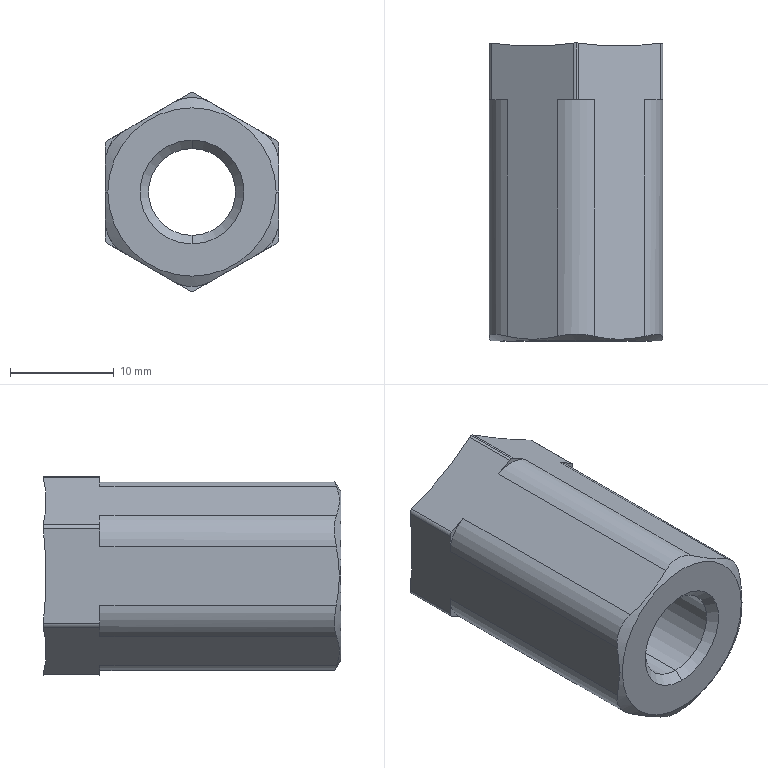Part | STEP file | _CMAZ40-N_a_n | 1 solid | 36 faces | box 16.7 x 28.679 x 19.129 mm | volume 5122 mm3 | cylinder 16 | plane 13 | cone 6 | spline 1 | commonest cylinder face diameters 1 x7 7 x7 8.376 x2
STEP:
#1=CARTESIAN_POINT('',(0.,4.188,4.188));
#2=VERTEX_POINT('',#1);
#3=CARTESIAN_POINT('',(0.,4.188,-4.188));
#4=VERTEX_POINT('',#3);
#5=CARTESIAN_POINT('',(0.,4.188,0.));
#6=DIRECTION('',(0.,-1.,0.));
#7=DIRECTION('',(0.,0.,-1.));
#8=AXIS2_PLACEMENT_3D('',#5,#6,#7);
#9=CIRCLE('',#8,4.188);
#10=EDGE_CURVE('',#2,#4,#9,.T.);
#11=ORIENTED_EDGE('',*,*,#10,.F.);
#12=CARTESIAN_POINT('',(0.,-22.388,4.188));
#13=VERTEX_POINT('',#12);
#14=CARTESIAN_POINT('',(0.,5.,4.188));
#15=DIRECTION('',(0.,-1.,0.));
#16=VECTOR('',#15,1000.);
#17=LINE('',#14,#16);
#18=EDGE_CURVE('',#2,#13,#17,.T.);
#19=ORIENTED_EDGE('',*,*,#18,.T.);
#20=CARTESIAN_POINT('',(0.,-22.388,-4.188));
#21=VERTEX_POINT('',#20);
#22=CARTESIAN_POINT('',(0.,-22.388,0.));
#23=DIRECTION('',(0.,1.,0.));
#24=DIRECTION('',(0.,0.,-1.));
#25=AXIS2_PLACEMENT_3D('',#22,#23,#24);
#26=CIRCLE('',#25,4.188);
#27=EDGE_CURVE('',#21,#13,#26,.T.);
#28=ORIENTED_EDGE('',*,*,#27,.F.);
#29=CARTESIAN_POINT('',(0.,5.,-4.188));
#30=DIRECTION('',(0.,-1.,0.));
#31=VECTOR('',#30,1000.);
#32=LINE('',#29,#31);
#33=EDGE_CURVE('',#4,#21,#32,.T.);
#34=ORIENTED_EDGE('',*,*,#33,.F.);
#35=EDGE_LOOP('',(#11,#19,#28,#34));
#36=FACE_OUTER_BOUND('',#35,.T.);
#37=CARTESIAN_POINT('',(0.,5.,0.));
#38=DIRECTION('',(0.,-1.,0.));
#39=DIRECTION('',(0.,0.,-1.));
#40=AXIS2_PLACEMENT_3D('',#37,#38,#39);
#41=CYLINDRICAL_SURFACE('',#40,4.188);
#42=ADVANCED_FACE('',(#36),#41,.F.);
#43=ORIENTED_EDGE('',*,*,#27,.T.);
#44=CARTESIAN_POINT('',(0.,-23.2,5.));
#45=VERTEX_POINT('',#44);
#46=CARTESIAN_POINT('',(0.,-23.2,5.));
#47=DIRECTION('',(0.,-0.7071,0.7071));
#48=VECTOR('',#47,1000.);
#49=LINE('',#46,#48);
#50=EDGE_CURVE('',#13,#45,#49,.T.);
#51=ORIENTED_EDGE('',*,*,#50,.T.);
#52=CARTESIAN_POINT('',(0.,-23.2,-5.));
#53=VERTEX_POINT('',#52);
#54=CARTESIAN_POINT('',(0.,-23.2,0.));
#55=DIRECTION('',(0.,1.,0.));
#56=DIRECTION('',(0.,0.,-1.));
#57=AXIS2_PLACEMENT_3D('',#54,#55,#56);
#58=CIRCLE('',#57,5.);
#59=EDGE_CURVE('',#53,#45,#58,.T.);
#60=ORIENTED_EDGE('',*,*,#59,.F.);
#61=CARTESIAN_POINT('',(0.,-23.2,-5.));
#62=DIRECTION('',(0.,-0.7071,-0.7071));
#63=VECTOR('',#62,1000.);
#64=LINE('',#61,#63);
#65=EDGE_CURVE('',#21,#53,#64,.T.);
#66=ORIENTED_EDGE('',*,*,#65,.F.);
#67=EDGE_LOOP('',(#43,#51,#60,#66));
#68=FACE_OUTER_BOUND('',#67,.T.);
#69=CARTESIAN_POINT('',(0.,-23.2,0.));
#70=DIRECTION('',(0.,-1.,0.));
#71=DIRECTION('',(0.,0.,-1.));
#72=AXIS2_PLACEMENT_3D('',#69,#70,#71);
#73=CONICAL_SURFACE('',#72,5.,0.7854);
#74=ADVANCED_FACE('',(#68),#73,.F.);
#75=ORIENTED_EDGE('',*,*,#10,.T.);
#76=CARTESIAN_POINT('',(0.,4.476,-4.476));
#77=VERTEX_POINT('',#76);
#78=CARTESIAN_POINT('',(0.,4.476,-4.476));
#79=DIRECTION('',(0.,0.7071,-0.7071));
#80=VECTOR('',#79,1000.);
#81=LINE('',#78,#80);
#82=EDGE_CURVE('',#4,#77,#81,.T.);
#83=ORIENTED_EDGE('',*,*,#82,.T.);
#84=CARTESIAN_POINT('',(0.,4.476,4.476));
#85=VERTEX_POINT('',#84);
#86=CARTESIAN_POINT('',(0.,4.476,0.));
#87=DIRECTION('',(0.,-1.,0.));
#88=DIRECTION('',(0.,0.,1.));
#89=AXIS2_PLACEMENT_3D('',#86,#87,#88);
#90=CIRCLE('',#89,4.476);
#91=EDGE_CURVE('',#85,#77,#90,.T.);
#92=ORIENTED_EDGE('',*,*,#91,.F.);
#93=CARTESIAN_POINT('',(0.,4.476,4.476));
#94=DIRECTION('',(0.,0.7071,0.7071));
#95=VECTOR('',#94,1000.);
#96=LINE('',#93,#95);
#97=EDGE_CURVE('',#2,#85,#96,.T.);
#98=ORIENTED_EDGE('',*,*,#97,.F.);
#99=EDGE_LOOP('',(#75,#83,#92,#98));
#100=FACE_OUTER_BOUND('',#99,.T.);
#101=CARTESIAN_POINT('',(0.,4.476,0.));
#102=DIRECTION('',(0.,1.,0.));
#103=DIRECTION('',(0.,0.,1.));
#104=AXIS2_PLACEMENT_3D('',#101,#102,#103);
#105=CONICAL_SURFACE('',#104,4.476,0.7854);
#106=ADVANCED_FACE('',(#100),#105,.F.);
#107=CARTESIAN_POINT('',(-8.1,-23.2,0.));
#108=VERTEX_POINT('',#107);
#109=CARTESIAN_POINT('',(8.1,-23.2,0.));
#110=VERTEX_POINT('',#109);
#111=CARTESIAN_POINT('',(0.,-23.2,0.));
#112=DIRECTION('',(0.,1.,0.));
#113=DIRECTION('',(-1.,0.,0.));
#114=AXIS2_PLACEMENT_3D('',#111,#112,#113);
#115=CIRCLE('',#114,8.1);
#116=EDGE_CURVE('',#108,#110,#115,.T.);
#117=ORIENTED_EDGE('',*,*,#116,.T.);
#118=CARTESIAN_POINT('',(8.35,-23.044,0.));
#119=VERTEX_POINT('',#118);
#120=CARTESIAN_POINT('',(9.106,-22.571,0.));
#121=DIRECTION('',(0.8481,0.5298,0.));
#122=VECTOR('',#121,1000.);
#123=LINE('',#120,#122);
#124=EDGE_CURVE('',#110,#119,#123,.T.);
#125=ORIENTED_EDGE('',*,*,#124,.T.);
#126=CARTESIAN_POINT('',(8.35,-22.758,2.8));
#127=VERTEX_POINT('',#126);
#128=CARTESIAN_POINT('',(8.35,-23.044,0.));
#129=CARTESIAN_POINT('',(8.35,-23.044,0.466));
#130=CARTESIAN_POINT('',(8.35,-23.019,0.9327));
#131=CARTESIAN_POINT('',(8.35,-22.923,1.867));
#132=CARTESIAN_POINT('',(8.35,-22.85,2.336));
#133=CARTESIAN_POINT('',(8.35,-22.758,2.8));
#134=B_SPLINE_CURVE_WITH_KNOTS('',3,(#128,#129,#130,#131,#132,#133),.UNSPECIFIED.,.F.,.F.,(4,2,4),(0.002807,0.004205,0.005602),.UNSPECIFIED.);
#135=EDGE_CURVE('',#119,#127,#134,.T.);
#136=ORIENTED_EDGE('',*,*,#135,.T.);
#137=CARTESIAN_POINT('',(6.6,-22.758,5.831));
#138=VERTEX_POINT('',#137);
#139=CARTESIAN_POINT('',(8.35,-22.758,2.8));
#140=CARTESIAN_POINT('',(8.35,-22.698,3.104));
#141=CARTESIAN_POINT('',(8.311,-22.653,3.404));
#142=CARTESIAN_POINT('',(8.193,-22.606,3.848));
#143=CARTESIAN_POINT('',(8.143,-22.595,3.995));
#144=CARTESIAN_POINT('',(8.026,-22.579,4.278));
#145=CARTESIAN_POINT('',(7.959,-22.575,4.416));
#146=CARTESIAN_POINT('',(7.729,-22.575,4.813));
#147=CARTESIAN_POINT('',(7.539,-22.591,5.062));
#148=CARTESIAN_POINT('',(7.108,-22.652,5.492));
#149=CARTESIAN_POINT('',(6.863,-22.698,5.679));
#150=CARTESIAN_POINT('',(6.6,-22.758,5.831));
#151=B_SPLINE_CURVE_WITH_KNOTS('',3,(#139,#140,#141,#142,#143,#144,#145,#146,#147,#148,#149,#150),.UNSPECIFIED.,.F.,.F.,(4,2,2,2,2,4),(0.,0.0009173,0.001376,0.001835,0.002752,0.003669),.UNSPECIFIED.);
#152=EDGE_CURVE('',#127,#138,#151,.T.);
#153=ORIENTED_EDGE('',*,*,#152,.T.);
#154=CARTESIAN_POINT('',(1.75,-22.758,8.631));
#155=VERTEX_POINT('',#154);
#156=CARTESIAN_POINT('',(6.6,-22.758,5.831));
#157=CARTESIAN_POINT('',(5.796,-22.943,6.296));
#158=CARTESIAN_POINT('',(4.989,-23.043,6.761));
#159=CARTESIAN_POINT('',(3.776,-23.044,7.462));
#160=CARTESIAN_POINT('',(3.371,-23.02,7.696));
#161=CARTESIAN_POINT('',(2.559,-22.923,8.164));
#162=CARTESIAN_POINT('',(2.153,-22.851,8.399));
#163=CARTESIAN_POINT('',(1.75,-22.758,8.631));
#164=B_SPLINE_CURVE_WITH_KNOTS('',3,(#156,#157,#158,#159,#160,#161,#162,#163),.UNSPECIFIED.,.F.,.F.,(4,2,2,4),(0.,0.002801,0.004202,0.005602),.UNSPECIFIED.);
#165=EDGE_CURVE('',#138,#155,#164,.T.);
#166=ORIENTED_EDGE('',*,*,#165,.T.);
#167=CARTESIAN_POINT('',(-1.75,-22.758,8.631));
#168=VERTEX_POINT('',#167);
#169=CARTESIAN_POINT('',(1.75,-22.758,8.631));
#170=CARTESIAN_POINT('',(1.487,-22.698,8.783));
#171=CARTESIAN_POINT('',(1.207,-22.653,8.9));
#172=CARTESIAN_POINT('',(0.7641,-22.606,9.019));
#173=CARTESIAN_POINT('',(0.6117,-22.595,9.05));
#174=CARTESIAN_POINT('',(0.3078,-22.579,9.09));
#175=CARTESIAN_POINT('',(0.1553,-22.575,9.1));
#176=CARTESIAN_POINT('',(-0.3037,-22.575,9.101));
#177=CARTESIAN_POINT('',(-0.6142,-22.591,9.059));
#178=CARTESIAN_POINT('',(-1.202,-22.652,8.901));
#179=CARTESIAN_POINT('',(-1.487,-22.698,8.783));
#180=CARTESIAN_POINT('',(-1.75,-22.758,8.631));
#181=B_SPLINE_CURVE_WITH_KNOTS('',3,(#169,#170,#171,#172,#173,#174,#175,#176,#177,#178,#179,#180),.UNSPECIFIED.,.F.,.F.,(4,2,2,2,2,4),(0.,0.0009173,0.001376,0.001835,0.002752,0.003669),.UNSPECIFIED.);
#182=EDGE_CURVE('',#155,#168,#181,.T.);
#183=ORIENTED_EDGE('',*,*,#182,.T.);
#184=CARTESIAN_POINT('',(-6.6,-22.758,5.831));
#185=VERTEX_POINT('',#184);
#186=CARTESIAN_POINT('',(-1.75,-22.758,8.631));
#187=CARTESIAN_POINT('',(-2.554,-22.943,8.167));
#188=CARTESIAN_POINT('',(-3.361,-23.043,7.701));
#189=CARTESIAN_POINT('',(-4.574,-23.044,7.001));
#190=CARTESIAN_POINT('',(-4.979,-23.02,6.767));
#191=CARTESIAN_POINT('',(-5.791,-22.923,6.299));
#192=CARTESIAN_POINT('',(-6.197,-22.851,6.064));
#193=CARTESIAN_POINT('',(-6.6,-22.758,5.831));
#194=B_SPLINE_CURVE_WITH_KNOTS('',3,(#186,#187,#188,#189,#190,#191,#192,#193),.UNSPECIFIED.,.F.,.F.,(4,2,2,4),(0.,0.002801,0.004202,0.005602),.UNSPECIFIED.);
#195=EDGE_CURVE('',#168,#185,#194,.T.);
#196=ORIENTED_EDGE('',*,*,#195,.T.);
#197=CARTESIAN_POINT('',(-8.35,-22.758,2.8));
#198=VERTEX_POINT('',#197);
#199=CARTESIAN_POINT('',(-6.6,-22.758,5.831));
#200=CARTESIAN_POINT('',(-6.863,-22.698,5.679));
#201=CARTESIAN_POINT('',(-7.104,-22.653,5.495));
#202=CARTESIAN_POINT('',(-7.429,-22.606,5.171));
#203=CARTESIAN_POINT('',(-7.532,-22.595,5.055));
#204=CARTESIAN_POINT('',(-7.718,-22.579,4.812));
#205=CARTESIAN_POINT('',(-7.803,-22.575,4.685));
#206=CARTESIAN_POINT('',(-8.033,-22.575,4.287));
#207=CARTESIAN_POINT('',(-8.153,-22.591,3.998));
#208=CARTESIAN_POINT('',(-8.31,-22.652,3.41));
#209=CARTESIAN_POINT('',(-8.35,-22.698,3.104));
#210=CARTESIAN_POINT('',(-8.35,-22.758,2.8));
#211=B_SPLINE_CURVE_WITH_KNOTS('',3,(#199,#200,#201,#202,#203,#204,#205,#206,#207,#208,#209,#210),.UNSPECIFIED.,.F.,.F.,(4,2,2,2,2,4),(0.,0.0009173,0.001376,0.001835,0.002752,0.003669),.UNSPECIFIED.);
#212=EDGE_CURVE('',#185,#198,#211,.T.);
#213=ORIENTED_EDGE('',*,*,#212,.T.);
#214=CARTESIAN_POINT('',(-8.35,-23.044,0.));
#215=VERTEX_POINT('',#214);
#216=CARTESIAN_POINT('',(-8.35,-22.758,2.8));
#217=CARTESIAN_POINT('',(-8.35,-22.943,1.869));
#218=CARTESIAN_POINT('',(-8.35,-23.044,0.936));
#219=CARTESIAN_POINT('',(-8.35,-23.044,0.));
#220=B_SPLINE_CURVE_WITH_KNOTS('',3,(#216,#217,#218,#219),.UNSPECIFIED.,.F.,.F.,(4,4),(0.,0.002807),.UNSPECIFIED.);
#221=EDGE_CURVE('',#198,#215,#220,.T.);
#222=ORIENTED_EDGE('',*,*,#221,.T.);
#223=CARTESIAN_POINT('',(-9.106,-22.571,0.));
#224=DIRECTION('',(-0.8481,0.5298,0.));
#225=VECTOR('',#224,1000.);
#226=LINE('',#223,#225);
#227=EDGE_CURVE('',#108,#215,#226,.T.);
#228=ORIENTED_EDGE('',*,*,#227,.F.);
#229=EDGE_LOOP('',(#117,#125,#136,#153,#166,#183,#196,#213,#222,#228));
#230=FACE_OUTER_BOUND('',#229,.T.);
#231=CARTESIAN_POINT('',(0.,-22.571,0.));
#232=DIRECTION('',(0.,1.,0.));
#233=DIRECTION('',(-1.,0.,0.));
#234=AXIS2_PLACEMENT_3D('',#231,#232,#233);
#235=CONICAL_SURFACE('',#234,9.106,1.012);
#236=ADVANCED_FACE('',(#230),#235,.T.);
#237=CARTESIAN_POINT('',(-1.75,0.,-8.631));
#238=VERTEX_POINT('',#237);
#239=CARTESIAN_POINT('',(0.,0.,-9.1));
#240=VERTEX_POINT('',#239);
#241=CARTESIAN_POINT('',(0.,0.,-5.6));
#242=DIRECTION('',(0.,-1.,0.));
#243=DIRECTION('',(0.,0.,-1.));
#244=AXIS2_PLACEMENT_3D('',#241,#242,#243);
#245=CIRCLE('',#244,3.5);
#246=EDGE_CURVE('',#238,#240,#245,.T.);
#247=ORIENTED_EDGE('',*,*,#246,.T.);
#248=CARTESIAN_POINT('',(0.,-22.575,-9.1));
#249=VERTEX_POINT('',#248);
#250=CARTESIAN_POINT('',(0.,-23.2,-9.1));
#251=DIRECTION('',(0.,-1.,0.));
#252=VECTOR('',#251,1000.);
#253=LINE('',#250,#252);
#254=EDGE_CURVE('',#240,#249,#253,.T.);
#255=ORIENTED_EDGE('',*,*,#254,.T.);
#256=CARTESIAN_POINT('',(-1.75,-22.758,-8.631));
#257=VERTEX_POINT('',#256);
#258=CARTESIAN_POINT('',(-1.75,-22.758,-8.631));
#259=CARTESIAN_POINT('',(-1.486,-22.698,-8.784));
#260=CARTESIAN_POINT('',(-1.207,-22.653,-8.9));
#261=CARTESIAN_POINT('',(-0.7628,-22.606,-9.02));
#262=CARTESIAN_POINT('',(-0.6101,-22.594,-9.05));
#263=CARTESIAN_POINT('',(-0.3059,-22.579,-9.09));
#264=CARTESIAN_POINT('',(-0.1532,-22.575,-9.1));
#265=CARTESIAN_POINT('',(0.,-22.575,-9.1));
#266=B_SPLINE_CURVE_WITH_KNOTS('',3,(#258,#259,#260,#261,#262,#263,#264,#265),.UNSPECIFIED.,.F.,.F.,(4,2,2,4),(0.,0.0009185,0.001378,0.001837),.UNSPECIFIED.);
#267=EDGE_CURVE('',#257,#249,#266,.T.);
#268=ORIENTED_EDGE('',*,*,#267,.F.);
#269=CARTESIAN_POINT('',(-1.75,-23.2,-8.631));
#270=DIRECTION('',(0.,-1.,0.));
#271=VECTOR('',#270,1000.);
#272=LINE('',#269,#271);
#273=EDGE_CURVE('',#238,#257,#272,.T.);
#274=ORIENTED_EDGE('',*,*,#273,.F.);
#275=EDGE_LOOP('',(#247,#255,#268,#274));
#276=FACE_OUTER_BOUND('',#275,.T.);
#277=CARTESIAN_POINT('',(0.,-23.2,-5.6));
#278=DIRECTION('',(0.,-1.,0.));
#279=DIRECTION('',(0.,0.,-1.));
#280=AXIS2_PLACEMENT_3D('',#277,#278,#279);
#281=CYLINDRICAL_SURFACE('',#280,3.5);
#282=ADVANCED_FACE('',(#276),#281,.T.);
#283=CARTESIAN_POINT('',(-0.25,0.,9.497));
#284=VERTEX_POINT('',#283);
#285=CARTESIAN_POINT('',(0.,0.,9.564));
#286=VERTEX_POINT('',#285);
#287=CARTESIAN_POINT('',(0.,0.,9.064));
#288=DIRECTION('',(0.,1.,0.));
#289=DIRECTION('',(0.,0.,1.));
#290=AXIS2_PLACEMENT_3D('',#287,#288,#289);
#291=CIRCLE('',#290,0.5);
#292=EDGE_CURVE('',#284,#286,#291,.T.);
#293=ORIENTED_EDGE('',*,*,#292,.T.);
#294=CARTESIAN_POINT('',(0.,5.479,9.564));
#295=VERTEX_POINT('',#294);
#296=CARTESIAN_POINT('',(0.,5.5,9.564));
#297=DIRECTION('',(0.,1.,0.));
#298=VECTOR('',#297,1000.);
#299=LINE('',#296,#298);
#300=EDGE_CURVE('',#286,#295,#299,.T.);
#301=ORIENTED_EDGE('',*,*,#300,.T.);
#302=CARTESIAN_POINT('',(-0.25,5.462,9.497));
#303=VERTEX_POINT('',#302);
#304=CARTESIAN_POINT('',(0.,5.479,9.564));
#305=CARTESIAN_POINT('',(-0.087,5.479,9.564));
#306=CARTESIAN_POINT('',(-0.1742,5.473,9.541));
#307=CARTESIAN_POINT('',(-0.25,5.462,9.497));
#308=B_SPLINE_CURVE_WITH_KNOTS('',3,(#304,#305,#306,#307),.UNSPECIFIED.,.F.,.F.,(4,4),(0.0002614,0.0005224),.UNSPECIFIED.);
#309=EDGE_CURVE('',#295,#303,#308,.T.);
#310=ORIENTED_EDGE('',*,*,#309,.T.);
#311=CARTESIAN_POINT('',(-0.25,-23.2,9.497));
#312=DIRECTION('',(0.,1.,0.));
#313=VECTOR('',#312,1000.);
#314=LINE('',#311,#313);
#315=EDGE_CURVE('',#284,#303,#314,.T.);
#316=ORIENTED_EDGE('',*,*,#315,.F.);
#317=EDGE_LOOP('',(#293,#301,#310,#316));
#318=FACE_OUTER_BOUND('',#317,.T.);
#319=CARTESIAN_POINT('',(0.,5.5,9.064));
#320=DIRECTION('',(0.,1.,0.));
#321=DIRECTION('',(0.,0.,1.));
#322=AXIS2_PLACEMENT_3D('',#319,#320,#321);
#323=CYLINDRICAL_SURFACE('',#322,0.5);
#324=ADVANCED_FACE('',(#318),#323,.T.);
#325=ORIENTED_EDGE('',*,*,#18,.F.);
#326=CARTESIAN_POINT('',(0.,4.188,0.));
#327=DIRECTION('',(0.,-1.,0.));
#328=DIRECTION('',(0.,0.,-1.));
#329=AXIS2_PLACEMENT_3D('',#326,#327,#328);
#330=CIRCLE('',#329,4.188);
#331=EDGE_CURVE('',#4,#2,#330,.T.);
#332=ORIENTED_EDGE('',*,*,#331,.F.);
#333=ORIENTED_EDGE('',*,*,#33,.T.);
#334=CARTESIAN_POINT('',(0.,-22.388,0.));
#335=DIRECTION('',(0.,1.,0.));
#336=DIRECTION('',(0.,0.,-1.));
#337=AXIS2_PLACEMENT_3D('',#334,#335,#336);
#338=CIRCLE('',#337,4.188);
#339=EDGE_CURVE('',#13,#21,#338,.T.);
#340=ORIENTED_EDGE('',*,*,#339,.F.);
#341=EDGE_LOOP('',(#325,#332,#333,#340));
#342=FACE_OUTER_BOUND('',#341,.T.);
#343=CARTESIAN_POINT('',(0.,5.,0.));
#344=DIRECTION('',(0.,-1.,0.));
#345=DIRECTION('',(0.,0.,-1.));
#346=AXIS2_PLACEMENT_3D('',#343,#344,#345);
#347=CYLINDRICAL_SURFACE('',#346,4.188);
#348=ADVANCED_FACE('',(#342),#347,.F.);
#349=ORIENTED_EDGE('',*,*,#50,.F.);
#350=ORIENTED_EDGE('',*,*,#339,.T.);
#351=ORIENTED_EDGE('',*,*,#65,.T.);
#352=CARTESIAN_POINT('',(0.,-23.2,0.));
#353=DIRECTION('',(0.,1.,0.));
#354=DIRECTION('',(0.,0.,-1.));
#355=AXIS2_PLACEMENT_3D('',#352,#353,#354);
#356=CIRCLE('',#355,5.);
#357=EDGE_CURVE('',#45,#53,#356,.T.);
#358=ORIENTED_EDGE('',*,*,#357,.F.);
#359=EDGE_LOOP('',(#349,#350,#351,#358));
#360=FACE_OUTER_BOUND('',#359,.T.);
#361=CARTESIAN_POINT('',(0.,-23.2,0.));
#362=DIRECTION('',(0.,-1.,0.));
#363=DIRECTION('',(0.,0.,-1.));
#364=AXIS2_PLACEMENT_3D('',#361,#362,#363);
#365=CONICAL_SURFACE('',#364,5.,0.7854);
#366=ADVANCED_FACE('',(#360),#365,.F.);
#367=ORIENTED_EDGE('',*,*,#82,.F.);
#368=ORIENTED_EDGE('',*,*,#331,.T.);
#369=ORIENTED_EDGE('',*,*,#97,.T.);
#370=CARTESIAN_POINT('',(0.,4.476,0.));
#371=DIRECTION('',(0.,-1.,0.));
#372=DIRECTION('',(0.,0.,1.));
#373=AXIS2_PLACEMENT_3D('',#370,#371,#372);
#374=CIRCLE('',#373,4.476);
#375=EDGE_CURVE('',#77,#85,#374,.T.);
#376=ORIENTED_EDGE('',*,*,#375,.F.);
#377=EDGE_LOOP('',(#367,#368,#369,#376));
#378=FACE_OUTER_BOUND('',#377,.T.);
#379=CARTESIAN_POINT('',(0.,4.476,0.));
#380=DIRECTION('',(0.,1.,0.));
#381=DIRECTION('',(0.,0.,1.));
#382=AXIS2_PLACEMENT_3D('',#379,#380,#381);
#383=CONICAL_SURFACE('',#382,4.476,0.7854);
#384=ADVANCED_FACE('',(#378),#383,.F.);
#385=ORIENTED_EDGE('',*,*,#59,.T.);
#386=ORIENTED_EDGE('',*,*,#357,.T.);
#387=EDGE_LOOP('',(#385,#386));
#388=FACE_BOUND('',#387,.T.);
#389=ORIENTED_EDGE('',*,*,#116,.F.);
#390=CARTESIAN_POINT('',(0.,-23.2,0.));
#391=DIRECTION('',(0.,1.,0.));
#392=DIRECTION('',(-1.,0.,0.));
#393=AXIS2_PLACEMENT_3D('',#390,#391,#392);
#394=CIRCLE('',#393,8.1);
#395=EDGE_CURVE('',#110,#108,#394,.T.);
#396=ORIENTED_EDGE('',*,*,#395,.F.);
#397=EDGE_LOOP('',(#389,#396));
#398=FACE_OUTER_BOUND('',#397,.T.);
#399=CARTESIAN_POINT('',(-4.85,-23.2,-2.8));
#400=DIRECTION('',(0.,1.,0.));
#401=DIRECTION('',(0.,0.,1.));
#402=AXIS2_PLACEMENT_3D('',#399,#400,#401);
#403=PLANE('',#402);
#404=ADVANCED_FACE('',(#388,#398),#403,.F.);
#405=CARTESIAN_POINT('',(0.25,5.462,9.497));
#406=VERTEX_POINT('',#405);
#407=CARTESIAN_POINT('',(0.25,5.462,9.497));
#408=CARTESIAN_POINT('',(0.1741,5.473,9.541));
#409=CARTESIAN_POINT('',(0.08716,5.479,9.564));
#410=CARTESIAN_POINT('',(0.,5.479,9.564));
#411=B_SPLINE_CURVE_WITH_KNOTS('',3,(#407,#408,#409,#410),.UNSPECIFIED.,.F.,.F.,(4,4),(0.,0.0002614),.UNSPECIFIED.);
#412=EDGE_CURVE('',#406,#295,#411,.T.);
#413=ORIENTED_EDGE('',*,*,#412,.F.);
#414=CARTESIAN_POINT('',(8.1,5.462,4.965));
#415=VERTEX_POINT('',#414);
#416=CARTESIAN_POINT('',(8.1,5.462,4.965));
#417=CARTESIAN_POINT('',(6.792,5.267,5.721));
#418=CARTESIAN_POINT('',(4.175,5.074,7.231));
#419=CARTESIAN_POINT('',(1.558,5.267,8.742));
#420=CARTESIAN_POINT('',(0.25,5.462,9.497));
#421=B_SPLINE_CURVE_WITH_KNOTS('',3,(#416,#417,#418,#419,#420),.UNSPECIFIED.,.F.,.F.,(4,1,4),(0.,0.004532,0.009064),.UNSPECIFIED.);
#422=EDGE_CURVE('',#415,#406,#421,.T.);
#423=ORIENTED_EDGE('',*,*,#422,.F.);
#424=CARTESIAN_POINT('',(8.35,5.462,4.532));
#425=VERTEX_POINT('',#424);
#426=CARTESIAN_POINT('',(8.35,5.462,4.532));
#427=CARTESIAN_POINT('',(8.35,5.473,4.62));
#428=CARTESIAN_POINT('',(8.327,5.479,4.707));
#429=CARTESIAN_POINT('',(8.24,5.479,4.857));
#430=CARTESIAN_POINT('',(8.176,5.473,4.921));
#431=CARTESIAN_POINT('',(8.1,5.462,4.965));
#432=B_SPLINE_CURVE_WITH_KNOTS('',3,(#426,#427,#428,#429,#430,#431),.UNSPECIFIED.,.F.,.F.,(4,2,4),(0.,0.0002612,0.0005224),.UNSPECIFIED.);
#433=EDGE_CURVE('',#425,#415,#432,.T.);
#434=ORIENTED_EDGE('',*,*,#433,.F.);
#435=CARTESIAN_POINT('',(8.35,5.462,-4.532));
#436=VERTEX_POINT('',#435);
#437=CARTESIAN_POINT('',(8.35,5.462,-4.532));
#438=CARTESIAN_POINT('',(8.35,5.267,-3.021));
#439=CARTESIAN_POINT('',(8.35,5.074,0.));
#440=CARTESIAN_POINT('',(8.35,5.267,3.021));
#441=CARTESIAN_POINT('',(8.35,5.462,4.532));
#442=B_SPLINE_CURVE_WITH_KNOTS('',3,(#437,#438,#439,#440,#441),.UNSPECIFIED.,.F.,.F.,(4,1,4),(0.,0.004532,0.009064),.UNSPECIFIED.);
#443=EDGE_CURVE('',#436,#425,#442,.T.);
#444=ORIENTED_EDGE('',*,*,#443,.F.);
#445=CARTESIAN_POINT('',(8.1,5.462,-4.965));
#446=VERTEX_POINT('',#445);
#447=CARTESIAN_POINT('',(8.1,5.462,-4.965));
#448=CARTESIAN_POINT('',(8.176,5.473,-4.921));
#449=CARTESIAN_POINT('',(8.239,5.479,-4.858));
#450=CARTESIAN_POINT('',(8.326,5.479,-4.707));
#451=CARTESIAN_POINT('',(8.35,5.473,-4.62));
#452=CARTESIAN_POINT('',(8.35,5.462,-4.532));
#453=B_SPLINE_CURVE_WITH_KNOTS('',3,(#447,#448,#449,#450,#451,#452),.UNSPECIFIED.,.F.,.F.,(4,2,4),(0.,0.0002612,0.0005224),.UNSPECIFIED.);
#454=EDGE_CURVE('',#446,#436,#453,.T.);
#455=ORIENTED_EDGE('',*,*,#454,.F.);
#456=CARTESIAN_POINT('',(0.25,5.462,-9.497));
#457=VERTEX_POINT('',#456);
#458=CARTESIAN_POINT('',(0.25,5.462,-9.497));
#459=CARTESIAN_POINT('',(1.558,5.267,-8.742));
#460=CARTESIAN_POINT('',(4.175,5.074,-7.231));
#461=CARTESIAN_POINT('',(6.792,5.267,-5.721));
#462=CARTESIAN_POINT('',(8.1,5.462,-4.965));
#463=B_SPLINE_CURVE_WITH_KNOTS('',3,(#458,#459,#460,#461,#462),.UNSPECIFIED.,.F.,.F.,(4,1,4),(0.,0.004532,0.009064),.UNSPECIFIED.);
#464=EDGE_CURVE('',#457,#446,#463,.T.);
#465=ORIENTED_EDGE('',*,*,#464,.F.);
#466=CARTESIAN_POINT('',(-0.25,5.462,-9.497));
#467=VERTEX_POINT('',#466);
#468=CARTESIAN_POINT('',(-0.25,5.462,-9.497));
#469=CARTESIAN_POINT('',(-0.1742,5.473,-9.541));
#470=CARTESIAN_POINT('',(-0.08731,5.479,-9.564));
#471=CARTESIAN_POINT('',(0.08685,5.479,-9.564));
#472=CARTESIAN_POINT('',(0.1742,5.473,-9.541));
#473=CARTESIAN_POINT('',(0.25,5.462,-9.497));
#474=B_SPLINE_CURVE_WITH_KNOTS('',3,(#468,#469,#470,#471,#472,#473),.UNSPECIFIED.,.F.,.F.,(4,2,4),(0.,0.0002612,0.0005224),.UNSPECIFIED.);
#475=EDGE_CURVE('',#467,#457,#474,.T.);
#476=ORIENTED_EDGE('',*,*,#475,.F.);
#477=CARTESIAN_POINT('',(-8.1,5.462,-4.965));
#478=VERTEX_POINT('',#477);
#479=CARTESIAN_POINT('',(-8.1,5.462,-4.965));
#480=CARTESIAN_POINT('',(-6.792,5.267,-5.721));
#481=CARTESIAN_POINT('',(-4.175,5.074,-7.231));
#482=CARTESIAN_POINT('',(-1.558,5.267,-8.742));
#483=CARTESIAN_POINT('',(-0.25,5.462,-9.497));
#484=B_SPLINE_CURVE_WITH_KNOTS('',3,(#479,#480,#481,#482,#483),.UNSPECIFIED.,.F.,.F.,(4,1,4),(0.,0.004532,0.009064),.UNSPECIFIED.);
#485=EDGE_CURVE('',#478,#467,#484,.T.);
#486=ORIENTED_EDGE('',*,*,#485,.F.);
#487=CARTESIAN_POINT('',(-8.35,5.462,-4.532));
#488=VERTEX_POINT('',#487);
#489=CARTESIAN_POINT('',(-8.35,5.462,-4.532));
#490=CARTESIAN_POINT('',(-8.35,5.473,-4.62));
#491=CARTESIAN_POINT('',(-8.327,5.479,-4.707));
#492=CARTESIAN_POINT('',(-8.24,5.479,-4.857));
#493=CARTESIAN_POINT('',(-8.176,5.473,-4.921));
#494=CARTESIAN_POINT('',(-8.1,5.462,-4.965));
#495=B_SPLINE_CURVE_WITH_KNOTS('',3,(#489,#490,#491,#492,#493,#494),.UNSPECIFIED.,.F.,.F.,(4,2,4),(0.,0.0002612,0.0005224),.UNSPECIFIED.);
#496=EDGE_CURVE('',#488,#478,#495,.T.);
#497=ORIENTED_EDGE('',*,*,#496,.F.);
#498=CARTESIAN_POINT('',(-8.35,5.462,4.532));
#499=VERTEX_POINT('',#498);
#500=CARTESIAN_POINT('',(-8.35,5.462,4.532));
#501=CARTESIAN_POINT('',(-8.35,5.267,3.021));
#502=CARTESIAN_POINT('',(-8.35,5.074,0.));
#503=CARTESIAN_POINT('',(-8.35,5.267,-3.021));
#504=CARTESIAN_POINT('',(-8.35,5.462,-4.532));
#505=B_SPLINE_CURVE_WITH_KNOTS('',3,(#500,#501,#502,#503,#504),.UNSPECIFIED.,.F.,.F.,(4,1,4),(0.,0.004532,0.009064),.UNSPECIFIED.);
#506=EDGE_CURVE('',#499,#488,#505,.T.);
#507=ORIENTED_EDGE('',*,*,#506,.F.);
#508=CARTESIAN_POINT('',(-8.1,5.462,4.965));
#509=VERTEX_POINT('',#508);
#510=CARTESIAN_POINT('',(-8.1,5.462,4.965));
#511=CARTESIAN_POINT('',(-8.176,5.473,4.921));
#512=CARTESIAN_POINT('',(-8.239,5.479,4.858));
#513=CARTESIAN_POINT('',(-8.326,5.479,4.707));
#514=CARTESIAN_POINT('',(-8.35,5.473,4.62));
#515=CARTESIAN_POINT('',(-8.35,5.462,4.532));
#516=B_SPLINE_CURVE_WITH_KNOTS('',3,(#510,#511,#512,#513,#514,#515),.UNSPECIFIED.,.F.,.F.,(4,2,4),(0.,0.0002612,0.0005224),.UNSPECIFIED.);
#517=EDGE_CURVE('',#509,#499,#516,.T.);
#518=ORIENTED_EDGE('',*,*,#517,.F.);
#519=CARTESIAN_POINT('',(-0.25,5.462,9.497));
#520=CARTESIAN_POINT('',(-1.558,5.267,8.742));
#521=CARTESIAN_POINT('',(-4.175,5.074,7.231));
#522=CARTESIAN_POINT('',(-6.792,5.267,5.721));
#523=CARTESIAN_POINT('',(-8.1,5.462,4.965));
#524=B_SPLINE_CURVE_WITH_KNOTS('',3,(#519,#520,#521,#522,#523),.UNSPECIFIED.,.F.,.F.,(4,1,4),(0.,0.004532,0.009064),.UNSPECIFIED.);
#525=EDGE_CURVE('',#303,#509,#524,.T.);
#526=ORIENTED_EDGE('',*,*,#525,.F.);
#527=ORIENTED_EDGE('',*,*,#309,.F.);
#528=EDGE_LOOP('',(#413,#423,#434,#444,#455,#465,#476,#486,#497,#507,#518,#526,#527));
#529=FACE_OUTER_BOUND('',#528,.T.);
#530=ORIENTED_EDGE('',*,*,#91,.T.);
#531=ORIENTED_EDGE('',*,*,#375,.T.);
#532=EDGE_LOOP('',(#530,#531));
#533=FACE_BOUND('',#532,.T.);
#534=CARTESIAN_POINT('',(-8.21,6.484,9.679));
#535=CARTESIAN_POINT('',(-2.788,5.18,9.679));
#536=CARTESIAN_POINT('',(2.788,5.18,9.679));
#537=CARTESIAN_POINT('',(8.21,6.484,9.679));
#538=CARTESIAN_POINT('',(-8.621,4.775,3.306));
#539=CARTESIAN_POINT('',(-2.928,3.405,3.306));
#540=CARTESIAN_POINT('',(2.928,3.405,3.306));
#541=CARTESIAN_POINT('',(8.621,4.775,3.306));
#542=CARTESIAN_POINT('',(-8.621,4.775,-3.306));
#543=CARTESIAN_POINT('',(-2.928,3.405,-3.306));
#544=CARTESIAN_POINT('',(2.928,3.405,-3.306));
#545=CARTESIAN_POINT('',(8.621,4.775,-3.306));
#546=CARTESIAN_POINT('',(-8.21,6.484,-9.679));
#547=CARTESIAN_POINT('',(-2.788,5.18,-9.679));
#548=CARTESIAN_POINT('',(2.788,5.18,-9.679));
#549=CARTESIAN_POINT('',(8.21,6.484,-9.679));
#550=(BOUNDED_SURFACE()B_SPLINE_SURFACE(3,3,((#534,#535,#536,#537),(#538,#539,#540,#541),(#542,#543,#544,#545),(#546,#547,#548,#549)),.UNSPECIFIED.,.F.,.F.,.F.)B_SPLINE_SURFACE_WITH_KNOTS((4,4),(4,4),(0.,1.),(0.,1.),.UNSPECIFIED.)GEOMETRIC_REPRESENTATION_ITEM()RATIONAL_B_SPLINE_SURFACE(((1.,0.9815,0.9815,1.),(0.976,0.9579,0.9579,0.976),(0.976,0.9579,0.9579,0.976),(1.,0.9815,0.9815,1.)))REPRESENTATION_ITEM('')SURFACE());
#551=ADVANCED_FACE('',(#529,#533),#550,.F.);
#552=ORIENTED_EDGE('',*,*,#124,.F.);
#553=ORIENTED_EDGE('',*,*,#395,.T.);
#554=ORIENTED_EDGE('',*,*,#227,.T.);
#555=CARTESIAN_POINT('',(-8.35,-22.758,-2.8));
#556=VERTEX_POINT('',#555);
#557=CARTESIAN_POINT('',(-8.35,-23.044,0.));
#558=CARTESIAN_POINT('',(-8.35,-23.044,-0.466));
#559=CARTESIAN_POINT('',(-8.35,-23.019,-0.9327));
#560=CARTESIAN_POINT('',(-8.35,-22.923,-1.867));
#561=CARTESIAN_POINT('',(-8.35,-22.85,-2.336));
#562=CARTESIAN_POINT('',(-8.35,-22.758,-2.8));
#563=B_SPLINE_CURVE_WITH_KNOTS('',3,(#557,#558,#559,#560,#561,#562),.UNSPECIFIED.,.F.,.F.,(4,2,4),(0.002807,0.004205,0.005602),.UNSPECIFIED.);
#564=EDGE_CURVE('',#215,#556,#563,.T.);
#565=ORIENTED_EDGE('',*,*,#564,.T.);
#566=CARTESIAN_POINT('',(-6.6,-22.758,-5.831));
#567=VERTEX_POINT('',#566);
#568=CARTESIAN_POINT('',(-8.35,-22.758,-2.8));
#569=CARTESIAN_POINT('',(-8.35,-22.698,-3.104));
#570=CARTESIAN_POINT('',(-8.311,-22.653,-3.404));
#571=CARTESIAN_POINT('',(-8.193,-22.606,-3.848));
#572=CARTESIAN_POINT('',(-8.143,-22.595,-3.995));
#573=CARTESIAN_POINT('',(-8.026,-22.579,-4.278));
#574=CARTESIAN_POINT('',(-7.959,-22.575,-4.416));
#575=CARTESIAN_POINT('',(-7.729,-22.575,-4.813));
#576=CARTESIAN_POINT('',(-7.539,-22.591,-5.062));
#577=CARTESIAN_POINT('',(-7.108,-22.652,-5.492));
#578=CARTESIAN_POINT('',(-6.863,-22.698,-5.679));
#579=CARTESIAN_POINT('',(-6.6,-22.758,-5.831));
#580=B_SPLINE_CURVE_WITH_KNOTS('',3,(#568,#569,#570,#571,#572,#573,#574,#575,#576,#577,#578,#579),.UNSPECIFIED.,.F.,.F.,(4,2,2,2,2,4),(0.,0.0009173,0.001376,0.001835,0.002752,0.003669),.UNSPECIFIED.);
#581=EDGE_CURVE('',#556,#567,#580,.T.);
#582=ORIENTED_EDGE('',*,*,#581,.T.);
#583=CARTESIAN_POINT('',(-6.6,-22.758,-5.831));
#584=CARTESIAN_POINT('',(-5.796,-22.943,-6.296));
#585=CARTESIAN_POINT('',(-4.989,-23.043,-6.761));
#586=CARTESIAN_POINT('',(-3.776,-23.044,-7.462));
#587=CARTESIAN_POINT('',(-3.371,-23.02,-7.696));
#588=CARTESIAN_POINT('',(-2.559,-22.923,-8.164));
#589=CARTESIAN_POINT('',(-2.153,-22.851,-8.399));
#590=CARTESIAN_POINT('',(-1.75,-22.758,-8.631));
#591=B_SPLINE_CURVE_WITH_KNOTS('',3,(#583,#584,#585,#586,#587,#588,#589,#590),.UNSPECIFIED.,.F.,.F.,(4,2,2,4),(0.,0.002801,0.004202,0.005602),.UNSPECIFIED.);
#592=EDGE_CURVE('',#567,#257,#591,.T.);
#593=ORIENTED_EDGE('',*,*,#592,.T.);
#594=ORIENTED_EDGE('',*,*,#267,.T.);
#595=CARTESIAN_POINT('',(1.75,-22.758,-8.631));
#596=VERTEX_POINT('',#595);
#597=CARTESIAN_POINT('',(0.,-22.575,-9.1));
#598=CARTESIAN_POINT('',(0.3056,-22.575,-9.1));
#599=CARTESIAN_POINT('',(0.6157,-22.591,-9.059));
#600=CARTESIAN_POINT('',(1.203,-22.652,-8.901));
#601=CARTESIAN_POINT('',(1.487,-22.698,-8.783));
#602=CARTESIAN_POINT('',(1.75,-22.758,-8.631));
#603=B_SPLINE_CURVE_WITH_KNOTS('',3,(#597,#598,#599,#600,#601,#602),.UNSPECIFIED.,.F.,.F.,(4,2,4),(0.001837,0.002753,0.003669),.UNSPECIFIED.);
#604=EDGE_CURVE('',#249,#596,#603,.T.);
#605=ORIENTED_EDGE('',*,*,#604,.T.);
#606=CARTESIAN_POINT('',(6.6,-22.758,-5.831));
#607=VERTEX_POINT('',#606);
#608=CARTESIAN_POINT('',(1.75,-22.758,-8.631));
#609=CARTESIAN_POINT('',(2.554,-22.943,-8.167));
#610=CARTESIAN_POINT('',(3.361,-23.043,-7.701));
#611=CARTESIAN_POINT('',(4.574,-23.044,-7.001));
#612=CARTESIAN_POINT('',(4.979,-23.02,-6.767));
#613=CARTESIAN_POINT('',(5.791,-22.923,-6.299));
#614=CARTESIAN_POINT('',(6.197,-22.851,-6.064));
#615=CARTESIAN_POINT('',(6.6,-22.758,-5.831));
#616=B_SPLINE_CURVE_WITH_KNOTS('',3,(#608,#609,#610,#611,#612,#613,#614,#615),.UNSPECIFIED.,.F.,.F.,(4,2,2,4),(0.,0.002801,0.004202,0.005602),.UNSPECIFIED.);
#617=EDGE_CURVE('',#596,#607,#616,.T.);
#618=ORIENTED_EDGE('',*,*,#617,.T.);
#619=CARTESIAN_POINT('',(8.35,-22.758,-2.8));
#620=VERTEX_POINT('',#619);
#621=CARTESIAN_POINT('',(6.6,-22.758,-5.831));
#622=CARTESIAN_POINT('',(6.863,-22.698,-5.679));
#623=CARTESIAN_POINT('',(7.104,-22.653,-5.495));
#624=CARTESIAN_POINT('',(7.429,-22.606,-5.171));
#625=CARTESIAN_POINT('',(7.532,-22.595,-5.055));
#626=CARTESIAN_POINT('',(7.718,-22.579,-4.812));
#627=CARTESIAN_POINT('',(7.803,-22.575,-4.685));
#628=CARTESIAN_POINT('',(8.033,-22.575,-4.287));
#629=CARTESIAN_POINT('',(8.153,-22.591,-3.998));
#630=CARTESIAN_POINT('',(8.31,-22.652,-3.41));
#631=CARTESIAN_POINT('',(8.35,-22.698,-3.104));
#632=CARTESIAN_POINT('',(8.35,-22.758,-2.8));
#633=B_SPLINE_CURVE_WITH_KNOTS('',3,(#621,#622,#623,#624,#625,#626,#627,#628,#629,#630,#631,#632),.UNSPECIFIED.,.F.,.F.,(4,2,2,2,2,4),(0.,0.0009173,0.001376,0.001835,0.002752,0.003669),.UNSPECIFIED.);
#634=EDGE_CURVE('',#607,#620,#633,.T.);
#635=ORIENTED_EDGE('',*,*,#634,.T.);
#636=CARTESIAN_POINT('',(8.35,-22.758,-2.8));
#637=CARTESIAN_POINT('',(8.35,-22.943,-1.869));
#638=CARTESIAN_POINT('',(8.35,-23.044,-0.936));
#639=CARTESIAN_POINT('',(8.35,-23.044,0.));
#640=B_SPLINE_CURVE_WITH_KNOTS('',3,(#636,#637,#638,#639),.UNSPECIFIED.,.F.,.F.,(4,4),(0.,0.002807),.UNSPECIFIED.);
#641=EDGE_CURVE('',#620,#119,#640,.T.);
#642=ORIENTED_EDGE('',*,*,#641,.T.);
#643=EDGE_LOOP('',(#552,#553,#554,#565,#582,#593,#594,#605,#618,#635,#642));
#644=FACE_OUTER_BOUND('',#643,.T.);
#645=CARTESIAN_POINT('',(0.,-22.571,0.));
#646=DIRECTION('',(0.,1.,0.));
#647=DIRECTION('',(-1.,0.,0.));
#648=AXIS2_PLACEMENT_3D('',#645,#646,#647);
#649=CONICAL_SURFACE('',#648,9.106,1.012);
#650=ADVANCED_FACE('',(#644),#649,.T.);
#651=CARTESIAN_POINT('',(-8.1,0.,4.965));
#652=VERTEX_POINT('',#651);
#653=CARTESIAN_POINT('',(-6.6,0.,5.831));
#654=VERTEX_POINT('',#653);
#655=CARTESIAN_POINT('',(-8.1,0.,4.965));
#656=DIRECTION('',(0.866,0.,0.5));
#657=VECTOR('',#656,1000.);
#658=LINE('',#655,#657);
#659=EDGE_CURVE('',#652,#654,#658,.T.);
#660=ORIENTED_EDGE('',*,*,#659,.T.);
#661=CARTESIAN_POINT('',(-6.6,-23.2,5.831));
#662=DIRECTION('',(0.,-1.,0.));
#663=VECTOR('',#662,1000.);
#664=LINE('',#661,#663);
#665=EDGE_CURVE('',#654,#185,#664,.T.);
#666=ORIENTED_EDGE('',*,*,#665,.T.);
#667=ORIENTED_EDGE('',*,*,#195,.F.);
#668=CARTESIAN_POINT('',(-1.75,0.,8.631));
#669=VERTEX_POINT('',#668);
#670=CARTESIAN_POINT('',(-1.75,-23.2,8.631));
#671=DIRECTION('',(0.,1.,0.));
#672=VECTOR('',#671,1000.);
#673=LINE('',#670,#672);
#674=EDGE_CURVE('',#168,#669,#673,.T.);
#675=ORIENTED_EDGE('',*,*,#674,.T.);
#676=CARTESIAN_POINT('',(-1.75,0.,8.631));
#677=DIRECTION('',(0.866,0.,0.5));
#678=VECTOR('',#677,1000.);
#679=LINE('',#676,#678);
#680=EDGE_CURVE('',#669,#284,#679,.T.);
#681=ORIENTED_EDGE('',*,*,#680,.T.);
#682=ORIENTED_EDGE('',*,*,#315,.T.);
#683=ORIENTED_EDGE('',*,*,#525,.T.);
#684=CARTESIAN_POINT('',(-8.1,-23.2,4.965));
#685=DIRECTION('',(0.,-1.,0.));
#686=VECTOR('',#685,1000.);
#687=LINE('',#684,#686);
#688=EDGE_CURVE('',#509,#652,#687,.T.);
#689=ORIENTED_EDGE('',*,*,#688,.T.);
#690=EDGE_LOOP('',(#660,#666,#667,#675,#681,#682,#683,#689));
#691=FACE_OUTER_BOUND('',#690,.T.);
#692=CARTESIAN_POINT('',(-6.6,-23.2,5.831));
#693=DIRECTION('',(-0.5,0.,0.866));
#694=DIRECTION('',(0.866,0.,0.5));
#695=AXIS2_PLACEMENT_3D('',#692,#693,#694);
#696=PLANE('',#695);
#697=ADVANCED_FACE('',(#691),#696,.T.);
#698=CARTESIAN_POINT('',(0.25,0.,9.497));
#699=VERTEX_POINT('',#698);
#700=CARTESIAN_POINT('',(1.75,0.,8.631));
#701=VERTEX_POINT('',#700);
#702=CARTESIAN_POINT('',(0.25,0.,9.497));
#703=DIRECTION('',(0.866,0.,-0.5));
#704=VECTOR('',#703,1000.);
#705=LINE('',#702,#704);
#706=EDGE_CURVE('',#699,#701,#705,.T.);
#707=ORIENTED_EDGE('',*,*,#706,.T.);
#708=CARTESIAN_POINT('',(1.75,-23.2,8.631));
#709=DIRECTION('',(0.,-1.,0.));
#710=VECTOR('',#709,1000.);
#711=LINE('',#708,#710);
#712=EDGE_CURVE('',#701,#155,#711,.T.);
#713=ORIENTED_EDGE('',*,*,#712,.T.);
#714=ORIENTED_EDGE('',*,*,#165,.F.);
#715=CARTESIAN_POINT('',(6.6,0.,5.831));
#716=VERTEX_POINT('',#715);
#717=CARTESIAN_POINT('',(6.6,-23.2,5.831));
#718=DIRECTION('',(0.,1.,0.));
#719=VECTOR('',#718,1000.);
#720=LINE('',#717,#719);
#721=EDGE_CURVE('',#138,#716,#720,.T.);
#722=ORIENTED_EDGE('',*,*,#721,.T.);
#723=CARTESIAN_POINT('',(8.1,0.,4.965));
#724=VERTEX_POINT('',#723);
#725=CARTESIAN_POINT('',(6.6,0.,5.831));
#726=DIRECTION('',(0.866,0.,-0.5));
#727=VECTOR('',#726,1000.);
#728=LINE('',#725,#727);
#729=EDGE_CURVE('',#716,#724,#728,.T.);
#730=ORIENTED_EDGE('',*,*,#729,.T.);
#731=CARTESIAN_POINT('',(8.1,-23.2,4.965));
#732=DIRECTION('',(0.,1.,0.));
#733=VECTOR('',#732,1000.);
#734=LINE('',#731,#733);
#735=EDGE_CURVE('',#724,#415,#734,.T.);
#736=ORIENTED_EDGE('',*,*,#735,.T.);
#737=ORIENTED_EDGE('',*,*,#422,.T.);
#738=CARTESIAN_POINT('',(0.25,-23.2,9.497));
#739=DIRECTION('',(0.,-1.,0.));
#740=VECTOR('',#739,1000.);
#741=LINE('',#738,#740);
#742=EDGE_CURVE('',#406,#699,#741,.T.);
#743=ORIENTED_EDGE('',*,*,#742,.T.);
#744=EDGE_LOOP('',(#707,#713,#714,#722,#730,#736,#737,#743));
#745=FACE_OUTER_BOUND('',#744,.T.);
#746=CARTESIAN_POINT('',(1.75,-23.2,8.631));
#747=DIRECTION('',(0.5,0.,0.866));
#748=DIRECTION('',(0.866,0.,-0.5));
#749=AXIS2_PLACEMENT_3D('',#746,#747,#748);
#750=PLANE('',#749);
#751=ADVANCED_FACE('',(#745),#750,.T.);
#752=CARTESIAN_POINT('',(8.35,0.,4.532));
#753=VERTEX_POINT('',#752);
#754=CARTESIAN_POINT('',(8.35,0.,2.8));
#755=VERTEX_POINT('',#754);
#756=CARTESIAN_POINT('',(8.35,0.,-4.532));
#757=DIRECTION('',(0.,0.,-1.));
#758=VECTOR('',#757,1000.);
#759=LINE('',#756,#758);
#760=EDGE_CURVE('',#753,#755,#759,.T.);
#761=ORIENTED_EDGE('',*,*,#760,.T.);
#762=CARTESIAN_POINT('',(8.35,-23.2,2.8));
#763=DIRECTION('',(0.,-1.,0.));
#764=VECTOR('',#763,1000.);
#765=LINE('',#762,#764);
#766=EDGE_CURVE('',#755,#127,#765,.T.);
#767=ORIENTED_EDGE('',*,*,#766,.T.);
#768=ORIENTED_EDGE('',*,*,#135,.F.);
#769=ORIENTED_EDGE('',*,*,#641,.F.);
#770=CARTESIAN_POINT('',(8.35,0.,-2.8));
#771=VERTEX_POINT('',#770);
#772=CARTESIAN_POINT('',(8.35,-23.2,-2.8));
#773=DIRECTION('',(0.,1.,0.));
#774=VECTOR('',#773,1000.);
#775=LINE('',#772,#774);
#776=EDGE_CURVE('',#620,#771,#775,.T.);
#777=ORIENTED_EDGE('',*,*,#776,.T.);
#778=CARTESIAN_POINT('',(8.35,0.,-4.532));
#779=VERTEX_POINT('',#778);
#780=CARTESIAN_POINT('',(8.35,0.,-4.532));
#781=DIRECTION('',(0.,0.,-1.));
#782=VECTOR('',#781,1000.);
#783=LINE('',#780,#782);
#784=EDGE_CURVE('',#771,#779,#783,.T.);
#785=ORIENTED_EDGE('',*,*,#784,.T.);
#786=CARTESIAN_POINT('',(8.35,-23.2,-4.532));
#787=DIRECTION('',(0.,1.,0.));
#788=VECTOR('',#787,1000.);
#789=LINE('',#786,#788);
#790=EDGE_CURVE('',#779,#436,#789,.T.);
#791=ORIENTED_EDGE('',*,*,#790,.T.);
#792=ORIENTED_EDGE('',*,*,#443,.T.);
#793=CARTESIAN_POINT('',(8.35,-23.2,4.532));
#794=DIRECTION('',(0.,-1.,0.));
#795=VECTOR('',#794,1000.);
#796=LINE('',#793,#795);
#797=EDGE_CURVE('',#425,#753,#796,.T.);
#798=ORIENTED_EDGE('',*,*,#797,.T.);
#799=EDGE_LOOP('',(#761,#767,#768,#769,#777,#785,#791,#792,#798));
#800=FACE_OUTER_BOUND('',#799,.T.);
#801=CARTESIAN_POINT('',(8.35,-23.2,2.8));
#802=DIRECTION('',(1.,0.,0.));
#803=DIRECTION('',(0.,0.,-1.));
#804=AXIS2_PLACEMENT_3D('',#801,#802,#803);
#805=PLANE('',#804);
#806=ADVANCED_FACE('',(#800),#805,.T.);
#807=CARTESIAN_POINT('',(8.1,0.,-4.965));
#808=VERTEX_POINT('',#807);
#809=CARTESIAN_POINT('',(6.6,0.,-5.831));
#810=VERTEX_POINT('',#809);
#811=CARTESIAN_POINT('',(8.1,0.,-4.965));
#812=DIRECTION('',(-0.866,0.,-0.5));
#813=VECTOR('',#812,1000.);
#814=LINE('',#811,#813);
#815=EDGE_CURVE('',#808,#810,#814,.T.);
#816=ORIENTED_EDGE('',*,*,#815,.T.);
#817=CARTESIAN_POINT('',(6.6,-23.2,-5.831));
#818=DIRECTION('',(0.,-1.,0.));
#819=VECTOR('',#818,1000.);
#820=LINE('',#817,#819);
#821=EDGE_CURVE('',#810,#607,#820,.T.);
#822=ORIENTED_EDGE('',*,*,#821,.T.);
#823=ORIENTED_EDGE('',*,*,#617,.F.);
#824=CARTESIAN_POINT('',(1.75,0.,-8.631));
#825=VERTEX_POINT('',#824);
#826=CARTESIAN_POINT('',(1.75,-23.2,-8.631));
#827=DIRECTION('',(0.,1.,0.));
#828=VECTOR('',#827,1000.);
#829=LINE('',#826,#828);
#830=EDGE_CURVE('',#596,#825,#829,.T.);
#831=ORIENTED_EDGE('',*,*,#830,.T.);
#832=CARTESIAN_POINT('',(0.25,0.,-9.497));
#833=VERTEX_POINT('',#832);
#834=CARTESIAN_POINT('',(1.75,0.,-8.631));
#835=DIRECTION('',(-0.866,0.,-0.5));
#836=VECTOR('',#835,1000.);
#837=LINE('',#834,#836);
#838=EDGE_CURVE('',#825,#833,#837,.T.);
#839=ORIENTED_EDGE('',*,*,#838,.T.);
#840=CARTESIAN_POINT('',(0.25,-23.2,-9.497));
#841=DIRECTION('',(0.,1.,0.));
#842=VECTOR('',#841,1000.);
#843=LINE('',#840,#842);
#844=EDGE_CURVE('',#833,#457,#843,.T.);
#845=ORIENTED_EDGE('',*,*,#844,.T.);
#846=ORIENTED_EDGE('',*,*,#464,.T.);
#847=CARTESIAN_POINT('',(8.1,-23.2,-4.965));
#848=DIRECTION('',(0.,-1.,0.));
#849=VECTOR('',#848,1000.);
#850=LINE('',#847,#849);
#851=EDGE_CURVE('',#446,#808,#850,.T.);
#852=ORIENTED_EDGE('',*,*,#851,.T.);
#853=EDGE_LOOP('',(#816,#822,#823,#831,#839,#845,#846,#852));
#854=FACE_OUTER_BOUND('',#853,.T.);
#855=CARTESIAN_POINT('',(6.6,-23.2,-5.831));
#856=DIRECTION('',(0.5,0.,-0.866));
#857=DIRECTION('',(-0.866,0.,-0.5));
#858=AXIS2_PLACEMENT_3D('',#855,#856,#857);
#859=PLANE('',#858);
#860=ADVANCED_FACE('',(#854),#859,.T.);
#861=CARTESIAN_POINT('',(-0.25,0.,-9.497));
#862=VERTEX_POINT('',#861);
#863=CARTESIAN_POINT('',(-0.25,0.,-9.497));
#864=DIRECTION('',(-0.866,0.,0.5));
#865=VECTOR('',#864,1000.);
#866=LINE('',#863,#865);
#867=EDGE_CURVE('',#862,#238,#866,.T.);
#868=ORIENTED_EDGE('',*,*,#867,.T.);
#869=ORIENTED_EDGE('',*,*,#273,.T.);
#870=ORIENTED_EDGE('',*,*,#592,.F.);
#871=CARTESIAN_POINT('',(-6.6,0.,-5.831));
#872=VERTEX_POINT('',#871);
#873=CARTESIAN_POINT('',(-6.6,-23.2,-5.831));
#874=DIRECTION('',(0.,1.,0.));
#875=VECTOR('',#874,1000.);
#876=LINE('',#873,#875);
#877=EDGE_CURVE('',#567,#872,#876,.T.);
#878=ORIENTED_EDGE('',*,*,#877,.T.);
#879=CARTESIAN_POINT('',(-8.1,0.,-4.965));
#880=VERTEX_POINT('',#879);
#881=CARTESIAN_POINT('',(-6.6,0.,-5.831));
#882=DIRECTION('',(-0.866,0.,0.5));
#883=VECTOR('',#882,1000.);
#884=LINE('',#881,#883);
#885=EDGE_CURVE('',#872,#880,#884,.T.);
#886=ORIENTED_EDGE('',*,*,#885,.T.);
#887=CARTESIAN_POINT('',(-8.1,-23.2,-4.965));
#888=DIRECTION('',(0.,1.,0.));
#889=VECTOR('',#888,1000.);
#890=LINE('',#887,#889);
#891=EDGE_CURVE('',#880,#478,#890,.T.);
#892=ORIENTED_EDGE('',*,*,#891,.T.);
#893=ORIENTED_EDGE('',*,*,#485,.T.);
#894=CARTESIAN_POINT('',(-0.25,-23.2,-9.497));
#895=DIRECTION('',(0.,-1.,0.));
#896=VECTOR('',#895,1000.);
#897=LINE('',#894,#896);
#898=EDGE_CURVE('',#467,#862,#897,.T.);
#899=ORIENTED_EDGE('',*,*,#898,.T.);
#900=EDGE_LOOP('',(#868,#869,#870,#878,#886,#892,#893,#899));
#901=FACE_OUTER_BOUND('',#900,.T.);
#902=CARTESIAN_POINT('',(-1.75,-23.2,-8.631));
#903=DIRECTION('',(-0.5,0.,-0.866));
#904=DIRECTION('',(-0.866,0.,0.5));
#905=AXIS2_PLACEMENT_3D('',#902,#903,#904);
#906=PLANE('',#905);
#907=ADVANCED_FACE('',(#901),#906,.T.);
#908=CARTESIAN_POINT('',(-8.35,0.,-4.532));
#909=VERTEX_POINT('',#908);
#910=CARTESIAN_POINT('',(-8.35,0.,-2.8));
#911=VERTEX_POINT('',#910);
#912=CARTESIAN_POINT('',(-8.35,0.,-4.532));
#913=DIRECTION('',(0.,0.,1.));
#914=VECTOR('',#913,1000.);
#915=LINE('',#912,#914);
#916=EDGE_CURVE('',#909,#911,#915,.T.);
#917=ORIENTED_EDGE('',*,*,#916,.T.);
#918=CARTESIAN_POINT('',(-8.35,-23.2,-2.8));
#919=DIRECTION('',(0.,-1.,0.));
#920=VECTOR('',#919,1000.);
#921=LINE('',#918,#920);
#922=EDGE_CURVE('',#911,#556,#921,.T.);
#923=ORIENTED_EDGE('',*,*,#922,.T.);
#924=ORIENTED_EDGE('',*,*,#564,.F.);
#925=ORIENTED_EDGE('',*,*,#221,.F.);
#926=CARTESIAN_POINT('',(-8.35,0.,2.8));
#927=VERTEX_POINT('',#926);
#928=CARTESIAN_POINT('',(-8.35,-23.2,2.8));
#929=DIRECTION('',(0.,1.,0.));
#930=VECTOR('',#929,1000.);
#931=LINE('',#928,#930);
#932=EDGE_CURVE('',#198,#927,#931,.T.);
#933=ORIENTED_EDGE('',*,*,#932,.T.);
#934=CARTESIAN_POINT('',(-8.35,0.,4.532));
#935=VERTEX_POINT('',#934);
#936=CARTESIAN_POINT('',(-8.35,0.,-4.532));
#937=DIRECTION('',(0.,0.,1.));
#938=VECTOR('',#937,1000.);
#939=LINE('',#936,#938);
#940=EDGE_CURVE('',#927,#935,#939,.T.);
#941=ORIENTED_EDGE('',*,*,#940,.T.);
#942=CARTESIAN_POINT('',(-8.35,-23.2,4.532));
#943=DIRECTION('',(0.,1.,0.));
#944=VECTOR('',#943,1000.);
#945=LINE('',#942,#944);
#946=EDGE_CURVE('',#935,#499,#945,.T.);
#947=ORIENTED_EDGE('',*,*,#946,.T.);
#948=ORIENTED_EDGE('',*,*,#506,.T.);
#949=CARTESIAN_POINT('',(-8.35,-23.2,-4.532));
#950=DIRECTION('',(0.,-1.,0.));
#951=VECTOR('',#950,1000.);
#952=LINE('',#949,#951);
#953=EDGE_CURVE('',#488,#909,#952,.T.);
#954=ORIENTED_EDGE('',*,*,#953,.T.);
#955=EDGE_LOOP('',(#917,#923,#924,#925,#933,#941,#947,#948,#954));
#956=FACE_OUTER_BOUND('',#955,.T.);
#957=CARTESIAN_POINT('',(-8.35,-23.2,-2.8));
#958=DIRECTION('',(-1.,0.,0.));
#959=DIRECTION('',(0.,0.,1.));
#960=AXIS2_PLACEMENT_3D('',#957,#958,#959);
#961=PLANE('',#960);
#962=ADVANCED_FACE('',(#956),#961,.T.);
#963=CARTESIAN_POINT('',(0.,0.,5.6));
#964=DIRECTION('',(0.,-1.,0.));
#965=DIRECTION('',(0.,0.,-1.));
#966=AXIS2_PLACEMENT_3D('',#963,#964,#965);
#967=CIRCLE('',#966,3.5);
#968=EDGE_CURVE('',#701,#669,#967,.T.);
#969=ORIENTED_EDGE('',*,*,#968,.T.);
#970=ORIENTED_EDGE('',*,*,#674,.F.);
#971=ORIENTED_EDGE('',*,*,#182,.F.);
#972=ORIENTED_EDGE('',*,*,#712,.F.);
#973=EDGE_LOOP('',(#969,#970,#971,#972));
#974=FACE_OUTER_BOUND('',#973,.T.);
#975=CARTESIAN_POINT('',(0.,-23.2,5.6));
#976=DIRECTION('',(0.,-1.,0.));
#977=DIRECTION('',(0.,0.,-1.));
#978=AXIS2_PLACEMENT_3D('',#975,#976,#977);
#979=CYLINDRICAL_SURFACE('',#978,3.5);
#980=ADVANCED_FACE('',(#974),#979,.T.);
#981=CARTESIAN_POINT('',(4.85,0.,2.8));
#982=DIRECTION('',(0.,-1.,0.));
#983=DIRECTION('',(0.,0.,-1.));
#984=AXIS2_PLACEMENT_3D('',#981,#982,#983);
#985=CIRCLE('',#984,3.5);
#986=EDGE_CURVE('',#755,#716,#985,.T.);
#987=ORIENTED_EDGE('',*,*,#986,.T.);
#988=ORIENTED_EDGE('',*,*,#721,.F.);
#989=ORIENTED_EDGE('',*,*,#152,.F.);
#990=ORIENTED_EDGE('',*,*,#766,.F.);
#991=EDGE_LOOP('',(#987,#988,#989,#990));
#992=FACE_OUTER_BOUND('',#991,.T.);
#993=CARTESIAN_POINT('',(4.85,-23.2,2.8));
#994=DIRECTION('',(0.,-1.,0.));
#995=DIRECTION('',(0.,0.,-1.));
#996=AXIS2_PLACEMENT_3D('',#993,#994,#995);
#997=CYLINDRICAL_SURFACE('',#996,3.5);
#998=ADVANCED_FACE('',(#992),#997,.T.);
#999=CARTESIAN_POINT('',(4.85,0.,-2.8));
#1000=DIRECTION('',(0.,-1.,0.));
#1001=DIRECTION('',(0.,0.,-1.));
#1002=AXIS2_PLACEMENT_3D('',#999,#1000,#1001);
#1003=CIRCLE('',#1002,3.5);
#1004=EDGE_CURVE('',#810,#771,#1003,.T.);
#1005=ORIENTED_EDGE('',*,*,#1004,.T.);
#1006=ORIENTED_EDGE('',*,*,#776,.F.);
#1007=ORIENTED_EDGE('',*,*,#634,.F.);
#1008=ORIENTED_EDGE('',*,*,#821,.F.);
#1009=EDGE_LOOP('',(#1005,#1006,#1007,#1008));
#1010=FACE_OUTER_BOUND('',#1009,.T.);
#1011=CARTESIAN_POINT('',(4.85,-23.2,-2.8));
#1012=DIRECTION('',(0.,-1.,0.));
#1013=DIRECTION('',(0.,0.,-1.));
#1014=AXIS2_PLACEMENT_3D('',#1011,#1012,#1013);
#1015=CYLINDRICAL_SURFACE('',#1014,3.5);
#1016=ADVANCED_FACE('',(#1010),#1015,.T.);
#1017=ORIENTED_EDGE('',*,*,#254,.F.);
#1018=CARTESIAN_POINT('',(0.,0.,-5.6));
#1019=DIRECTION('',(0.,-1.,0.));
#1020=DIRECTION('',(0.,0.,-1.));
#1021=AXIS2_PLACEMENT_3D('',#1018,#1019,#1020);
#1022=CIRCLE('',#1021,3.5);
#1023=EDGE_CURVE('',#240,#825,#1022,.T.);
#1024=ORIENTED_EDGE('',*,*,#1023,.T.);
#1025=ORIENTED_EDGE('',*,*,#830,.F.);
#1026=ORIENTED_EDGE('',*,*,#604,.F.);
#1027=EDGE_LOOP('',(#1017,#1024,#1025,#1026));
#1028=FACE_OUTER_BOUND('',#1027,.T.);
#1029=CARTESIAN_POINT('',(0.,-23.2,-5.6));
#1030=DIRECTION('',(0.,-1.,0.));
#1031=DIRECTION('',(0.,0.,-1.));
#1032=AXIS2_PLACEMENT_3D('',#1029,#1030,#1031);
#1033=CYLINDRICAL_SURFACE('',#1032,3.5);
#1034=ADVANCED_FACE('',(#1028),#1033,.T.);
#1035=CARTESIAN_POINT('',(-4.85,0.,-2.8));
#1036=DIRECTION('',(0.,-1.,0.));
#1037=DIRECTION('',(0.,0.,-1.));
#1038=AXIS2_PLACEMENT_3D('',#1035,#1036,#1037);
#1039=CIRCLE('',#1038,3.5);
#1040=EDGE_CURVE('',#911,#872,#1039,.T.);
#1041=ORIENTED_EDGE('',*,*,#1040,.T.);
#1042=ORIENTED_EDGE('',*,*,#877,.F.);
#1043=ORIENTED_EDGE('',*,*,#581,.F.);
#1044=ORIENTED_EDGE('',*,*,#922,.F.);
#1045=EDGE_LOOP('',(#1041,#1042,#1043,#1044));
#1046=FACE_OUTER_BOUND('',#1045,.T.);
#1047=CARTESIAN_POINT('',(-4.85,-23.2,-2.8));
#1048=DIRECTION('',(0.,-1.,0.));
#1049=DIRECTION('',(0.,0.,-1.));
#1050=AXIS2_PLACEMENT_3D('',#1047,#1048,#1049);
#1051=CYLINDRICAL_SURFACE('',#1050,3.5);
#1052=ADVANCED_FACE('',(#1046),#1051,.T.);
#1053=CARTESIAN_POINT('',(-4.85,0.,2.8));
#1054=DIRECTION('',(0.,-1.,0.));
#1055=DIRECTION('',(0.,0.,-1.));
#1056=AXIS2_PLACEMENT_3D('',#1053,#1054,#1055);
#1057=CIRCLE('',#1056,3.5);
#1058=EDGE_CURVE('',#654,#927,#1057,.T.);
#1059=ORIENTED_EDGE('',*,*,#1058,.T.);
#1060=ORIENTED_EDGE('',*,*,#932,.F.);
#1061=ORIENTED_EDGE('',*,*,#212,.F.);
#1062=ORIENTED_EDGE('',*,*,#665,.F.);
#1063=EDGE_LOOP('',(#1059,#1060,#1061,#1062));
#1064=FACE_OUTER_BOUND('',#1063,.T.);
#1065=CARTESIAN_POINT('',(-4.85,-23.2,2.8));
#1066=DIRECTION('',(0.,-1.,0.));
#1067=DIRECTION('',(0.,0.,-1.));
#1068=AXIS2_PLACEMENT_3D('',#1065,#1066,#1067);
#1069=CYLINDRICAL_SURFACE('',#1068,3.5);
#1070=ADVANCED_FACE('',(#1064),#1069,.T.);
#1071=ORIENTED_EDGE('',*,*,#946,.F.);
#1072=CARTESIAN_POINT('',(-7.85,0.,4.532));
#1073=DIRECTION('',(0.,1.,0.));
#1074=DIRECTION('',(0.,0.,1.));
#1075=AXIS2_PLACEMENT_3D('',#1072,#1073,#1074);
#1076=CIRCLE('',#1075,0.5);
#1077=EDGE_CURVE('',#935,#652,#1076,.T.);
#1078=ORIENTED_EDGE('',*,*,#1077,.T.);
#1079=ORIENTED_EDGE('',*,*,#688,.F.);
#1080=ORIENTED_EDGE('',*,*,#517,.T.);
#1081=EDGE_LOOP('',(#1071,#1078,#1079,#1080));
#1082=FACE_OUTER_BOUND('',#1081,.T.);
#1083=CARTESIAN_POINT('',(-7.85,5.5,4.532));
#1084=DIRECTION('',(0.,1.,0.));
#1085=DIRECTION('',(0.,0.,1.));
#1086=AXIS2_PLACEMENT_3D('',#1083,#1084,#1085);
#1087=CYLINDRICAL_SURFACE('',#1086,0.5);
#1088=ADVANCED_FACE('',(#1082),#1087,.T.);
#1089=ORIENTED_EDGE('',*,*,#300,.F.);
#1090=CARTESIAN_POINT('',(0.,0.,9.064));
#1091=DIRECTION('',(0.,1.,0.));
#1092=DIRECTION('',(0.,0.,1.));
#1093=AXIS2_PLACEMENT_3D('',#1090,#1091,#1092);
#1094=CIRCLE('',#1093,0.5);
#1095=EDGE_CURVE('',#286,#699,#1094,.T.);
#1096=ORIENTED_EDGE('',*,*,#1095,.T.);
#1097=ORIENTED_EDGE('',*,*,#742,.F.);
#1098=ORIENTED_EDGE('',*,*,#412,.T.);
#1099=EDGE_LOOP('',(#1089,#1096,#1097,#1098));
#1100=FACE_OUTER_BOUND('',#1099,.T.);
#1101=CARTESIAN_POINT('',(0.,5.5,9.064));
#1102=DIRECTION('',(0.,1.,0.));
#1103=DIRECTION('',(0.,0.,1.));
#1104=AXIS2_PLACEMENT_3D('',#1101,#1102,#1103);
#1105=CYLINDRICAL_SURFACE('',#1104,0.5);
#1106=ADVANCED_FACE('',(#1100),#1105,.T.);
#1107=ORIENTED_EDGE('',*,*,#735,.F.);
#1108=CARTESIAN_POINT('',(7.85,0.,4.532));
#1109=DIRECTION('',(0.,1.,0.));
#1110=DIRECTION('',(0.,0.,1.));
#1111=AXIS2_PLACEMENT_3D('',#1108,#1109,#1110);
#1112=CIRCLE('',#1111,0.5);
#1113=EDGE_CURVE('',#724,#753,#1112,.T.);
#1114=ORIENTED_EDGE('',*,*,#1113,.T.);
#1115=ORIENTED_EDGE('',*,*,#797,.F.);
#1116=ORIENTED_EDGE('',*,*,#433,.T.);
#1117=EDGE_LOOP('',(#1107,#1114,#1115,#1116));
#1118=FACE_OUTER_BOUND('',#1117,.T.);
#1119=CARTESIAN_POINT('',(7.85,5.5,4.532));
#1120=DIRECTION('',(0.,1.,0.));
#1121=DIRECTION('',(0.,0.,1.));
#1122=AXIS2_PLACEMENT_3D('',#1119,#1120,#1121);
#1123=CYLINDRICAL_SURFACE('',#1122,0.5);
#1124=ADVANCED_FACE('',(#1118),#1123,.T.);
#1125=ORIENTED_EDGE('',*,*,#790,.F.);
#1126=CARTESIAN_POINT('',(7.85,0.,-4.532));
#1127=DIRECTION('',(0.,1.,0.));
#1128=DIRECTION('',(0.,0.,1.));
#1129=AXIS2_PLACEMENT_3D('',#1126,#1127,#1128);
#1130=CIRCLE('',#1129,0.5);
#1131=EDGE_CURVE('',#779,#808,#1130,.T.);
#1132=ORIENTED_EDGE('',*,*,#1131,.T.);
#1133=ORIENTED_EDGE('',*,*,#851,.F.);
#1134=ORIENTED_EDGE('',*,*,#454,.T.);
#1135=EDGE_LOOP('',(#1125,#1132,#1133,#1134));
#1136=FACE_OUTER_BOUND('',#1135,.T.);
#1137=CARTESIAN_POINT('',(7.85,5.5,-4.532));
#1138=DIRECTION('',(0.,1.,0.));
#1139=DIRECTION('',(0.,0.,1.));
#1140=AXIS2_PLACEMENT_3D('',#1137,#1138,#1139);
#1141=CYLINDRICAL_SURFACE('',#1140,0.5);
#1142=ADVANCED_FACE('',(#1136),#1141,.T.);
#1143=ORIENTED_EDGE('',*,*,#844,.F.);
#1144=CARTESIAN_POINT('',(0.,0.,-9.064));
#1145=DIRECTION('',(0.,1.,0.));
#1146=DIRECTION('',(0.,0.,1.));
#1147=AXIS2_PLACEMENT_3D('',#1144,#1145,#1146);
#1148=CIRCLE('',#1147,0.5);
#1149=EDGE_CURVE('',#833,#862,#1148,.T.);
#1150=ORIENTED_EDGE('',*,*,#1149,.T.);
#1151=ORIENTED_EDGE('',*,*,#898,.F.);
#1152=ORIENTED_EDGE('',*,*,#475,.T.);
#1153=EDGE_LOOP('',(#1143,#1150,#1151,#1152));
#1154=FACE_OUTER_BOUND('',#1153,.T.);
#1155=CARTESIAN_POINT('',(0.,5.5,-9.064));
#1156=DIRECTION('',(0.,1.,0.));
#1157=DIRECTION('',(0.,0.,1.));
#1158=AXIS2_PLACEMENT_3D('',#1155,#1156,#1157);
#1159=CYLINDRICAL_SURFACE('',#1158,0.5);
#1160=ADVANCED_FACE('',(#1154),#1159,.T.);
#1161=ORIENTED_EDGE('',*,*,#891,.F.);
#1162=CARTESIAN_POINT('',(-7.85,0.,-4.532));
#1163=DIRECTION('',(0.,1.,0.));
#1164=DIRECTION('',(0.,0.,1.));
#1165=AXIS2_PLACEMENT_3D('',#1162,#1163,#1164);
#1166=CIRCLE('',#1165,0.5);
#1167=EDGE_CURVE('',#880,#909,#1166,.T.);
#1168=ORIENTED_EDGE('',*,*,#1167,.T.);
#1169=ORIENTED_EDGE('',*,*,#953,.F.);
#1170=ORIENTED_EDGE('',*,*,#496,.T.);
#1171=EDGE_LOOP('',(#1161,#1168,#1169,#1170));
#1172=FACE_OUTER_BOUND('',#1171,.T.);
#1173=CARTESIAN_POINT('',(-7.85,5.5,-4.532));
#1174=DIRECTION('',(0.,1.,0.));
#1175=DIRECTION('',(0.,0.,1.));
#1176=AXIS2_PLACEMENT_3D('',#1173,#1174,#1175);
#1177=CYLINDRICAL_SURFACE('',#1176,0.5);
#1178=ADVANCED_FACE('',(#1172),#1177,.T.);
#1179=ORIENTED_EDGE('',*,*,#968,.F.);
#1180=ORIENTED_EDGE('',*,*,#706,.F.);
#1181=ORIENTED_EDGE('',*,*,#1095,.F.);
#1182=ORIENTED_EDGE('',*,*,#292,.F.);
#1183=ORIENTED_EDGE('',*,*,#680,.F.);
#1184=EDGE_LOOP('',(#1179,#1180,#1181,#1182,#1183));
#1185=FACE_OUTER_BOUND('',#1184,.T.);
#1186=CARTESIAN_POINT('',(-7.85,0.,-4.532));
#1187=DIRECTION('',(0.,1.,0.));
#1188=DIRECTION('',(0.,0.,1.));
#1189=AXIS2_PLACEMENT_3D('',#1186,#1187,#1188);
#1190=PLANE('',#1189);
#1191=ADVANCED_FACE('',(#1185),#1190,.F.);
#1192=ORIENTED_EDGE('',*,*,#986,.F.);
#1193=ORIENTED_EDGE('',*,*,#760,.F.);
#1194=ORIENTED_EDGE('',*,*,#1113,.F.);
#1195=ORIENTED_EDGE('',*,*,#729,.F.);
#1196=EDGE_LOOP('',(#1192,#1193,#1194,#1195));
#1197=FACE_OUTER_BOUND('',#1196,.T.);
#1198=CARTESIAN_POINT('',(-7.85,0.,-4.532));
#1199=DIRECTION('',(0.,1.,0.));
#1200=DIRECTION('',(0.,0.,1.));
#1201=AXIS2_PLACEMENT_3D('',#1198,#1199,#1200);
#1202=PLANE('',#1201);
#1203=ADVANCED_FACE('',(#1197),#1202,.F.);
#1204=ORIENTED_EDGE('',*,*,#1004,.F.);
#1205=ORIENTED_EDGE('',*,*,#815,.F.);
#1206=ORIENTED_EDGE('',*,*,#1131,.F.);
#1207=ORIENTED_EDGE('',*,*,#784,.F.);
#1208=EDGE_LOOP('',(#1204,#1205,#1206,#1207));
#1209=FACE_OUTER_BOUND('',#1208,.T.);
#1210=CARTESIAN_POINT('',(-7.85,0.,-4.532));
#1211=DIRECTION('',(0.,1.,0.));
#1212=DIRECTION('',(0.,0.,1.));
#1213=AXIS2_PLACEMENT_3D('',#1210,#1211,#1212);
#1214=PLANE('',#1213);
#1215=ADVANCED_FACE('',(#1209),#1214,.F.);
#1216=ORIENTED_EDGE('',*,*,#246,.F.);
#1217=ORIENTED_EDGE('',*,*,#867,.F.);
#1218=ORIENTED_EDGE('',*,*,#1149,.F.);
#1219=ORIENTED_EDGE('',*,*,#838,.F.);
#1220=ORIENTED_EDGE('',*,*,#1023,.F.);
#1221=EDGE_LOOP('',(#1216,#1217,#1218,#1219,#1220));
#1222=FACE_OUTER_BOUND('',#1221,.T.);
#1223=CARTESIAN_POINT('',(-7.85,0.,-4.532));
#1224=DIRECTION('',(0.,1.,0.));
#1225=DIRECTION('',(0.,0.,1.));
#1226=AXIS2_PLACEMENT_3D('',#1223,#1224,#1225);
#1227=PLANE('',#1226);
#1228=ADVANCED_FACE('',(#1222),#1227,.F.);
#1229=ORIENTED_EDGE('',*,*,#1040,.F.);
#1230=ORIENTED_EDGE('',*,*,#916,.F.);
#1231=ORIENTED_EDGE('',*,*,#1167,.F.);
#1232=ORIENTED_EDGE('',*,*,#885,.F.);
#1233=EDGE_LOOP('',(#1229,#1230,#1231,#1232));
#1234=FACE_OUTER_BOUND('',#1233,.T.);
#1235=CARTESIAN_POINT('',(-7.85,0.,-4.532));
#1236=DIRECTION('',(0.,1.,0.));
#1237=DIRECTION('',(0.,0.,1.));
#1238=AXIS2_PLACEMENT_3D('',#1235,#1236,#1237);
#1239=PLANE('',#1238);
#1240=ADVANCED_FACE('',(#1234),#1239,.F.);
#1241=ORIENTED_EDGE('',*,*,#1058,.F.);
#1242=ORIENTED_EDGE('',*,*,#659,.F.);
#1243=ORIENTED_EDGE('',*,*,#1077,.F.);
#1244=ORIENTED_EDGE('',*,*,#940,.F.);
#1245=EDGE_LOOP('',(#1241,#1242,#1243,#1244));
#1246=FACE_OUTER_BOUND('',#1245,.T.);
#1247=CARTESIAN_POINT('',(-7.85,0.,-4.532));
#1248=DIRECTION('',(0.,1.,0.));
#1249=DIRECTION('',(0.,0.,1.));
#1250=AXIS2_PLACEMENT_3D('',#1247,#1248,#1249);
#1251=PLANE('',#1250);
#1252=ADVANCED_FACE('',(#1246),#1251,.F.);
#1253=CLOSED_SHELL('',(#42,#74,#106,#236,#282,#324,#348,#366,#384,#404,#551,#650,#697,#751,#806,#860,#907,#962,#980,#998,#1016,#1034,#1052,#1070,#1088,#1106,#1124,#1142,#1160,#1178,#1191,#1203,#1215,#1228,#1240,#1252));
#1254=MANIFOLD_SOLID_BREP('',#1253);
#1255=CARTESIAN_POINT('',(0.,0.,0.));
#1256=DIRECTION('',(0.,0.,1.));
#1257=DIRECTION('',(1.,0.,0.));
#1258=AXIS2_PLACEMENT_3D('',#1255,#1256,#1257);
#1259=(LENGTH_UNIT()NAMED_UNIT(*)SI_UNIT(.MILLI.,.METRE.));
#1260=UNCERTAINTY_MEASURE_WITH_UNIT(LENGTH_MEASURE(0.00001),#1259,'','');
#1261=(NAMED_UNIT(*)PLANE_ANGLE_UNIT()SI_UNIT($,.RADIAN.));
#1262=(NAMED_UNIT(*)SI_UNIT($,.STERADIAN.)SOLID_ANGLE_UNIT());
#1263=(GEOMETRIC_REPRESENTATION_CONTEXT(3)GLOBAL_UNCERTAINTY_ASSIGNED_CONTEXT((#1260))GLOBAL_UNIT_ASSIGNED_CONTEXT((#1259,#1261,#1262))REPRESENTATION_CONTEXT('',''));
#1264=ADVANCED_BREP_SHAPE_REPRESENTATION('',(#1254,#1258),#1263);